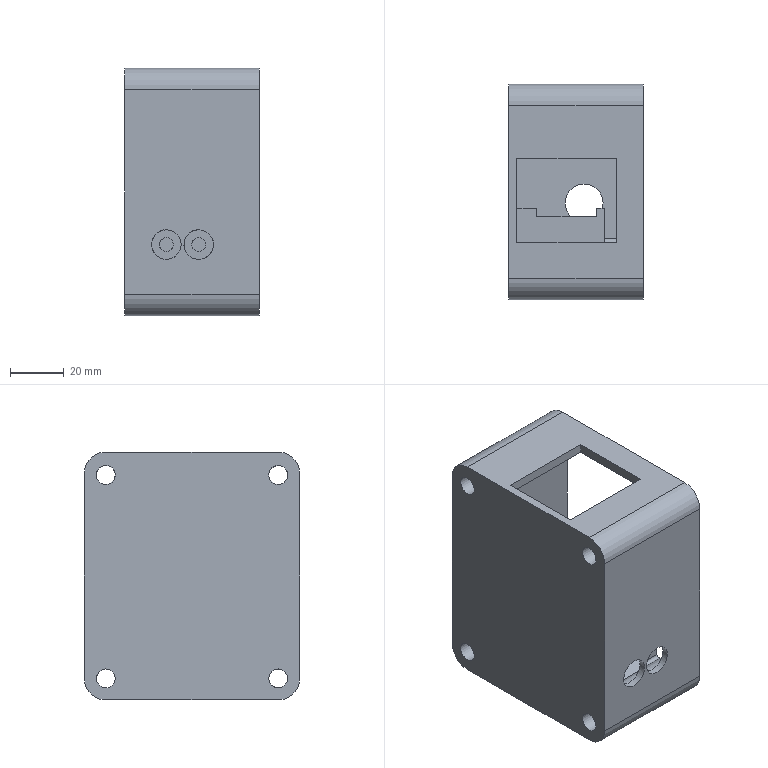NC program | NX | posted by the shop | part box 50 x 80 x 92 mm
Whole program:
%
O1234(4)
(T=7 D6-18-D6-50-3T-rough Z=-18.00 D=6.00 R=0.00 L=50.00)
(T=9 D2-6-D4-50-3T-rough Z=-6.00 D=2.00 R=0.00 L=7.00)
G40 G17 G80 G90 G21
M9
M5
G91 G28 Z0.0
M1
N1
(T=11 N=D6-18-D6-50-3T-rough D=1.00 R=0.00 FL=10.00 L=11.00)
(XY-STOCK=0.05)
T11 M6
T9
G0 G90 G54 X9.4 Y-7.861 S4500 M3
G43 H11 Z30.
M8
Z1.
G1 Y-6.1 Z.995 F1500.
X-15.9 Z.929
Y-36.9 Z.849
X9.4 Z.782
Y-6.1 Z.702
X-15.9 Z.635
Y-36.9 Z.555
X9.4 Z.489
Y-6.1 Z.408
X-15.9 Z.342
Y-36.9 Z.261
X9.4 Z.195
Y-6.1 Z.114
X-15.9 Z.048
Y-36.9 Z-.033
X9.4 Z-.099
Y-6.1 Z-.18
X-15.9 Z-.246
Y-36.9 Z-.326
X9.4 Z-.393
Y-6.1 Z-.473
X-15.9 Z-.54
Y-36.9 Z-.62
X9.4 Z-.686
Y-6.1 Z-.767
X-15.9 Z-.833
Y-36.9 Z-.914
X9.4 Z-.98
Y-6.1 Z-1.061
X-15.9 Z-1.127
Y-36.9 Z-1.208
X9.4 Z-1.274
Y-6.1 Z-1.355
X-15.9 Z-1.421
Y-36.9 Z-1.501
X9.4 Z-1.568
Y-6.1 Z-1.648
X-15.9 Z-1.715
Y-36.9 Z-1.795
X9.4 Z-1.861
Y-6.1 Z-1.942
X-15.9 Z-2.008
Y-36.9 Z-2.089
X9.4 Z-2.155
Y-6.1 Z-2.236
X-15.9 Z-2.302
Y-36.9 Z-2.383
X9.4 Z-2.449
Y-6.1 Z-2.529
X-15.9 Z-2.596
Y-36.9 Z-2.676
X9.4 Z-2.743
Y-6.1 Z-2.823
X-15.9 Z-2.889
Y-36.9 Z-2.97
X9.4 Z-3.036
Y-6.1 Z-3.117
X-15.9 Z-3.183
Y-36.9 Z-3.264
X9.4 Z-3.33
Y-6.1 Z-3.411
X-15.9 Z-3.477
Y-36.9 Z-3.558
X9.4 Z-3.624
Y-6.1 Z-3.704
X-15.9 Z-3.771
Y-36.9 Z-3.851
X9.4 Z-3.918
Y-6.1 Z-3.998
X-15.9 Z-4.064
Y-36.9 Z-4.145
X9.4 Z-4.211
Y-6.1 Z-4.292
X-15.9 Z-4.358
Y-36.9 Z-4.439
X9.4 Z-4.505
Y-6.1 Z-4.586
X-15.9 Z-4.652
Y-36.9 Z-4.733
X9.4 Z-4.799
Y-6.1 Z-4.879
X-15.9 Z-4.946
Y-36.9 Z-5.026
X9.4 Z-5.093
Y-6.1 Z-5.173
X-15.9 Z-5.239
Y-36.9 Z-5.32
X9.4 Z-5.386
Y-6.1 Z-5.467
X-3.25 Z-5.5
X-15.9
Y-36.9
X9.4
Y-6.1
X-3.25
Z-4.5
G0 Z30.
G0 X-1.25 Y-8. S4500 M3
M8
Z-6.5
G1 Z-8.5 F600.
G3 X-3.25 Y-6. I-2. J0.0
G1 X-16.
Y-37.
X9.5
Y-6.
X-3.25
G3 X-5.25 Y-8. I0.0 J-2.
G1 Z-6.5
G0 Z30.
M9
M5
G91 G28 Z0.0
M1
N2
(T=9 N=D2-6-D4-50-3T-rough D=2.00 R=0.00 FL=6.00 L=7.00)
(XY-STOCK=0.10)
T9 M6
T11
G0 G90 G54 X-12.394 Y-6.1 S4500 M3
G43 H09 Z30.
M8
Z1.5
G1 Z-.5 F600.
G3 X-14.394 Y-4.1 I-2. J0.0
G1 X-17.9
Y-7.606
G3 X-15.9 Y-9.606 I2. J0.0
G1 Z1.5
G0 X-12.394 Y-6.1 Z1.
G1 Z-1.
G3 X-14.394 Y-4.1 I-2. J0.0
G1 X-17.9
Y-7.606
G3 X-15.9 Y-9.606 I2. J0.0
G1 Z1.
G0 X-12.394 Y-6.1 Z.5
G1 Z-1.5
G3 X-14.394 Y-4.1 I-2. J0.0
G1 X-17.9
Y-7.606
G3 X-15.9 Y-9.606 I2. J0.0
G1 Z.5
G0 X-12.394 Y-6.1 Z0.0
G1 Z-2.
G3 X-14.394 Y-4.1 I-2. J0.0
G1 X-17.9
Y-7.606
G3 X-15.9 Y-9.606 I2. J0.0
G1 Z0.0
G0 X-12.394 Y-6.1 Z-.5
G1 Z-2.5
G3 X-14.394 Y-4.1 I-2. J0.0
G1 X-17.9
Y-7.606
G3 X-15.9 Y-9.606 I2. J0.0
G1 Z-.5
G0 X-12.394 Y-6.1 Z-1.
G1 Z-3.
G3 X-14.394 Y-4.1 I-2. J0.0
G1 X-17.9
Y-7.606
G3 X-15.9 Y-9.606 I2. J0.0
G1 Z-1.
G0 X-12.394 Y-6.1 Z-1.5
G1 Z-3.5
G3 X-14.394 Y-4.1 I-2. J0.0
G1 X-17.9
Y-7.606
G3 X-15.9 Y-9.606 I2. J0.0
G1 Z-1.5
G0 X-12.394 Y-6.1 Z-2.
G1 Z-4.
G3 X-14.394 Y-4.1 I-2. J0.0
G1 X-17.9
Y-7.606
G3 X-15.9 Y-9.606 I2. J0.0
G1 Z-2.
G0 X-12.394 Y-6.1 Z-2.5
G1 Z-4.5
G3 X-14.394 Y-4.1 I-2. J0.0
G1 X-17.9
Y-7.606
G3 X-15.9 Y-9.606 I2. J0.0
G1 Z-2.5
G0 X-12.394 Y-6.1 Z-3.
G1 Z-5.
G3 X-14.394 Y-4.1 I-2. J0.0
G1 X-17.9
Y-7.606
G3 X-15.9 Y-9.606 I2. J0.0
G1 Z-3.
G0 X-12.394 Y-6.1 Z-3.5
G1 Z-5.5
G3 X-14.394 Y-4.1 I-2. J0.0
G1 X-17.9
Y-7.606
G3 X-15.9 Y-9.606 I2. J0.0
G1 Z-3.5
G0 Z30.
X9.4
Z1.5
G1 Z-.5
G3 X11.4 Y-7.606 I0.0 J2.
G1 Y-4.1
X7.894
G3 X5.894 Y-6.1 I0.0 J-2.
G1 Z1.5
G0 X9.4 Y-9.606 Z1.
G1 Z-1.
G3 X11.4 Y-7.606 I0.0 J2.
G1 Y-4.1
X7.894
G3 X5.894 Y-6.1 I0.0 J-2.
G1 Z1.
G0 X9.4 Y-9.606 Z.5
G1 Z-1.5
G3 X11.4 Y-7.606 I0.0 J2.
G1 Y-4.1
X7.894
G3 X5.894 Y-6.1 I0.0 J-2.
G1 Z.5
G0 X9.4 Y-9.606 Z0.0
G1 Z-2.
G3 X11.4 Y-7.606 I0.0 J2.
G1 Y-4.1
X7.894
G3 X5.894 Y-6.1 I0.0 J-2.
G1 Z0.0
G0 X9.4 Y-9.606 Z-.5
G1 Z-2.5
G3 X11.4 Y-7.606 I0.0 J2.
G1 Y-4.1
X7.894
G3 X5.894 Y-6.1 I0.0 J-2.
G1 Z-.5
G0 X9.4 Y-9.606 Z-1.
G1 Z-3.
G3 X11.4 Y-7.606 I0.0 J2.
G1 Y-4.1
X7.894
G3 X5.894 Y-6.1 I0.0 J-2.
G1 Z-1.
G0 X9.4 Y-9.606 Z-1.5
G1 Z-3.5
G3 X11.4 Y-7.606 I0.0 J2.
G1 Y-4.1
X7.894
G3 X5.894 Y-6.1 I0.0 J-2.
G1 Z-1.5
G0 X9.4 Y-9.606 Z-2.
G1 Z-4.
G3 X11.4 Y-7.606 I0.0 J2.
G1 Y-4.1
X7.894
G3 X5.894 Y-6.1 I0.0 J-2.
G1 Z-2.
G0 X9.4 Y-9.606 Z-2.5
G1 Z-4.5
G3 X11.4 Y-7.606 I0.0 J2.
G1 Y-4.1
X7.894
G3 X5.894 Y-6.1 I0.0 J-2.
G1 Z-2.5
G0 X9.4 Y-9.606 Z-3.
G1 Z-5.
G3 X11.4 Y-7.606 I0.0 J2.
G1 Y-4.1
X7.894
G3 X5.894 Y-6.1 I0.0 J-2.
G1 Z-3.
G0 X9.4 Y-9.606 Z-3.5
G1 Z-5.5
G3 X11.4 Y-7.606 I0.0 J2.
G1 Y-4.1
X7.894
G3 X5.894 Y-6.1 I0.0 J-2.
G1 Z-3.5
G0 Z30.
Y-36.9
Z1.5
G1 Z-.5
G3 X7.894 Y-38.9 I2. J0.0
G1 X11.4
Y-35.394
G3 X9.4 Y-33.394 I-2. J0.0
G1 Z1.5
G0 X5.894 Y-36.9 Z1.
G1 Z-1.
G3 X7.894 Y-38.9 I2. J0.0
G1 X11.4
Y-35.394
G3 X9.4 Y-33.394 I-2. J0.0
G1 Z1.
G0 X5.894 Y-36.9 Z.5
G1 Z-1.5
G3 X7.894 Y-38.9 I2. J0.0
G1 X11.4
Y-35.394
G3 X9.4 Y-33.394 I-2. J0.0
G1 Z.5
G0 X5.894 Y-36.9 Z0.0
G1 Z-2.
G3 X7.894 Y-38.9 I2. J0.0
G1 X11.4
Y-35.394
G3 X9.4 Y-33.394 I-2. J0.0
G1 Z0.0
G0 X5.894 Y-36.9 Z-.5
G1 Z-2.5
G3 X7.894 Y-38.9 I2. J0.0
G1 X11.4
Y-35.394
G3 X9.4 Y-33.394 I-2. J0.0
G1 Z-.5
G0 X5.894 Y-36.9 Z-1.
G1 Z-3.
G3 X7.894 Y-38.9 I2. J0.0
G1 X11.4
Y-35.394
G3 X9.4 Y-33.394 I-2. J0.0
G1 Z-1.
G0 X5.894 Y-36.9 Z-1.5
G1 Z-3.5
G3 X7.894 Y-38.9 I2. J0.0
G1 X11.4
Y-35.394
G3 X9.4 Y-33.394 I-2. J0.0
G1 Z-1.5
G0 X5.894 Y-36.9 Z-2.
G1 Z-4.
G3 X7.894 Y-38.9 I2. J0.0
G1 X11.4
Y-35.394
G3 X9.4 Y-33.394 I-2. J0.0
G1 Z-2.
G0 X5.894 Y-36.9 Z-2.5
G1 Z-4.5
G3 X7.894 Y-38.9 I2. J0.0
G1 X11.4
Y-35.394
G3 X9.4 Y-33.394 I-2. J0.0
G1 Z-2.5
G0 X5.894 Y-36.9 Z-3.
G1 Z-5.
G3 X7.894 Y-38.9 I2. J0.0
G1 X11.4
Y-35.394
G3 X9.4 Y-33.394 I-2. J0.0
G1 Z-3.
G0 X5.894 Y-36.9 Z-3.5
G1 Z-5.5
G3 X7.894 Y-38.9 I2. J0.0
G1 X11.4
Y-35.394
G3 X9.4 Y-33.394 I-2. J0.0
G1 Z-3.5
G0 Z30.
X-15.9
Z1.5
G1 Z-.5
G3 X-17.9 Y-35.394 I0.0 J-2.
G1 Y-38.9
X-14.394
G3 X-12.394 Y-36.9 I0.0 J2.
G1 Z1.5
G0 X-15.9 Y-33.394 Z1.
G1 Z-1.
G3 X-17.9 Y-35.394 I0.0 J-2.
G1 Y-38.9
X-14.394
G3 X-12.394 Y-36.9 I0.0 J2.
G1 Z1.
G0 X-15.9 Y-33.394 Z.5
G1 Z-1.5
G3 X-17.9 Y-35.394 I0.0 J-2.
G1 Y-38.9
X-14.394
G3 X-12.394 Y-36.9 I0.0 J2.
G1 Z.5
G0 X-15.9 Y-33.394 Z0.0
G1 Z-2.
G3 X-17.9 Y-35.394 I0.0 J-2.
G1 Y-38.9
X-14.394
G3 X-12.394 Y-36.9 I0.0 J2.
G1 Z0.0
G0 X-15.9 Y-33.394 Z-.5
G1 Z-2.5
G3 X-17.9 Y-35.394 I0.0 J-2.
G1 Y-38.9
X-14.394
G3 X-12.394 Y-36.9 I0.0 J2.
G1 Z-.5
G0 X-15.9 Y-33.394 Z-1.
G1 Z-3.
G3 X-17.9 Y-35.394 I0.0 J-2.
G1 Y-38.9
X-14.394
G3 X-12.394 Y-36.9 I0.0 J2.
G1 Z-1.
G0 X-15.9 Y-33.394 Z-1.5
G1 Z-3.5
G3 X-17.9 Y-35.394 I0.0 J-2.
G1 Y-38.9
X-14.394
G3 X-12.394 Y-36.9 I0.0 J2.
G1 Z-1.5
G0 X-15.9 Y-33.394 Z-2.
G1 Z-4.
G3 X-17.9 Y-35.394 I0.0 J-2.
G1 Y-38.9
X-14.394
G3 X-12.394 Y-36.9 I0.0 J2.
G1 Z-2.
G0 X-15.9 Y-33.394 Z-2.5
G1 Z-4.5
G3 X-17.9 Y-35.394 I0.0 J-2.
G1 Y-38.9
X-14.394
G3 X-12.394 Y-36.9 I0.0 J2.
G1 Z-2.5
G0 X-15.9 Y-33.394 Z-3.
G1 Z-5.
G3 X-17.9 Y-35.394 I0.0 J-2.
G1 Y-38.9
X-14.394
G3 X-12.394 Y-36.9 I0.0 J2.
G1 Z-3.
G0 X-15.9 Y-33.394 Z-3.5
G1 Z-5.5
G3 X-17.9 Y-35.394 I0.0 J-2.
G1 Y-38.9
X-14.394
G3 X-12.394 Y-36.9 I0.0 J2.
G1 Z-3.5
G0 Z30.
M9
M5
G91 G28 Z0.0
G28 Y0.
M30
%